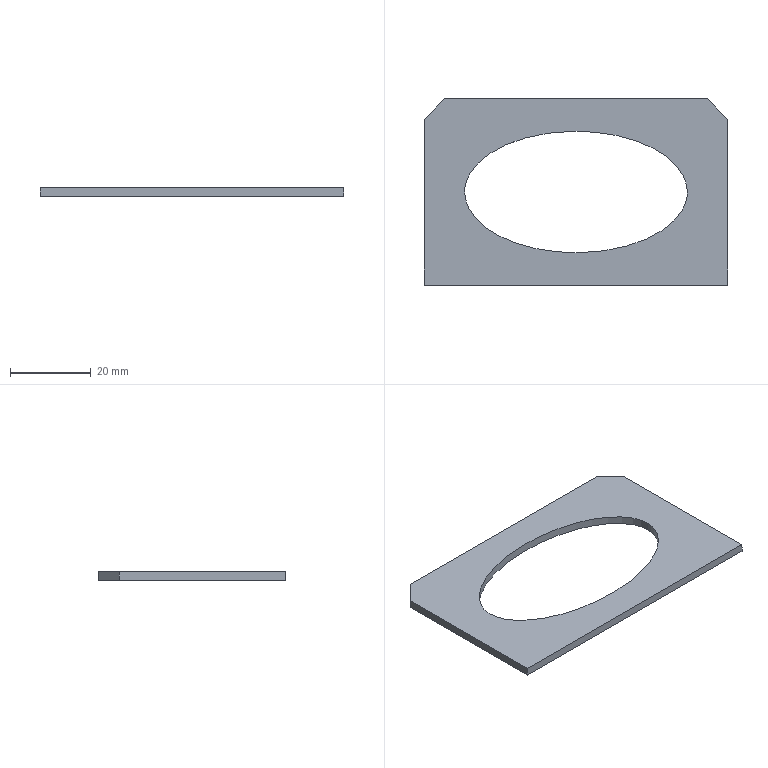Part | SolidWorks | features Chamfer 1, Cut 1, FlatPattern 1, SMBaseFlange 1, SheetMetal 1 | 1 solid | 10 faces | box 75 x 46 x 2 mm | volume 4258 mm3 | plane 8 | spline 2
STEP:
#1=CARTESIAN_POINT('',(27.5,0.,-2.));
#2=VERTEX_POINT('',#1);
#3=CARTESIAN_POINT('',(-27.5,0.,-2.));
#4=VERTEX_POINT('',#3);
#5=CARTESIAN_POINT('',(27.5,0.,-2.));
#6=CARTESIAN_POINT('',(27.5,30.,-2.));
#7=CARTESIAN_POINT('',(-27.5,30.,-2.));
#8=CARTESIAN_POINT('',(-27.5,0.,-2.));
#9=(BOUNDED_CURVE()B_SPLINE_CURVE(3,(#5,#6,#7,#8),.UNSPECIFIED.,.F.,.T.)B_SPLINE_CURVE_WITH_KNOTS((4,4),(3.142,6.283),.UNSPECIFIED.)CURVE()GEOMETRIC_REPRESENTATION_ITEM()RATIONAL_B_SPLINE_CURVE((1.,0.3333,0.3333,1.))REPRESENTATION_ITEM(''));
#10=EDGE_CURVE('',#2,#4,#9,.T.);
#11=ORIENTED_EDGE('',*,*,#10,.F.);
#12=CARTESIAN_POINT('',(27.5,0.,0.));
#13=VERTEX_POINT('',#12);
#14=CARTESIAN_POINT('',(27.5,0.,-2.));
#15=DIRECTION('',(0.,0.,1.));
#16=VECTOR('',#15,1000.);
#17=LINE('',#14,#16);
#18=EDGE_CURVE('',#2,#13,#17,.T.);
#19=ORIENTED_EDGE('',*,*,#18,.T.);
#20=CARTESIAN_POINT('',(-27.5,0.,0.));
#21=VERTEX_POINT('',#20);
#22=CARTESIAN_POINT('',(27.5,0.,0.));
#23=CARTESIAN_POINT('',(27.5,30.,0.));
#24=CARTESIAN_POINT('',(-27.5,30.,0.));
#25=CARTESIAN_POINT('',(-27.5,0.,0.));
#26=(BOUNDED_CURVE()B_SPLINE_CURVE(3,(#22,#23,#24,#25),.UNSPECIFIED.,.F.,.F.)B_SPLINE_CURVE_WITH_KNOTS((4,4),(3.142,6.283),.UNSPECIFIED.)CURVE()GEOMETRIC_REPRESENTATION_ITEM()RATIONAL_B_SPLINE_CURVE((1.,0.3333,0.3333,1.))REPRESENTATION_ITEM(''));
#27=EDGE_CURVE('',#13,#21,#26,.T.);
#28=ORIENTED_EDGE('',*,*,#27,.T.);
#29=CARTESIAN_POINT('',(-27.5,0.,-2.));
#30=DIRECTION('',(0.,0.,1.));
#31=VECTOR('',#30,1000.);
#32=LINE('',#29,#31);
#33=EDGE_CURVE('',#4,#21,#32,.T.);
#34=ORIENTED_EDGE('',*,*,#33,.F.);
#35=EDGE_LOOP('',(#11,#19,#28,#34));
#36=FACE_OUTER_BOUND('',#35,.T.);
#37=CARTESIAN_POINT('',(27.5,0.,-2.));
#38=CARTESIAN_POINT('',(27.5,0.,0.));
#39=CARTESIAN_POINT('',(27.5,30.,-2.));
#40=CARTESIAN_POINT('',(27.5,30.,0.));
#41=CARTESIAN_POINT('',(-27.5,30.,-2.));
#42=CARTESIAN_POINT('',(-27.5,30.,0.));
#43=CARTESIAN_POINT('',(-27.5,0.,-2.));
#44=CARTESIAN_POINT('',(-27.5,0.,0.));
#45=(BOUNDED_SURFACE()B_SPLINE_SURFACE(3,1,((#37,#38),(#39,#40),(#41,#42),(#43,#44)),.UNSPECIFIED.,.F.,.F.,.T.)B_SPLINE_SURFACE_WITH_KNOTS((4,4),(2,2),(0.,1.),(0.,1.),.UNSPECIFIED.)GEOMETRIC_REPRESENTATION_ITEM()RATIONAL_B_SPLINE_SURFACE(((1.,1.),(0.3333,0.3333),(0.3333,0.3333),(1.,1.)))REPRESENTATION_ITEM('')SURFACE());
#46=ADVANCED_FACE('',(#36),#45,.F.);
#47=CARTESIAN_POINT('',(37.5,-23.,-2.));
#48=VERTEX_POINT('',#47);
#49=CARTESIAN_POINT('',(37.5,18.,-2.));
#50=VERTEX_POINT('',#49);
#51=CARTESIAN_POINT('',(37.5,23.,-2.));
#52=DIRECTION('',(0.,1.,0.));
#53=VECTOR('',#52,1000.);
#54=LINE('',#51,#53);
#55=EDGE_CURVE('',#48,#50,#54,.T.);
#56=ORIENTED_EDGE('',*,*,#55,.T.);
#57=CARTESIAN_POINT('',(37.5,18.,0.));
#58=VERTEX_POINT('',#57);
#59=CARTESIAN_POINT('',(37.5,18.,-2.));
#60=DIRECTION('',(0.,0.,1.));
#61=VECTOR('',#60,1000.);
#62=LINE('',#59,#61);
#63=EDGE_CURVE('',#50,#58,#62,.T.);
#64=ORIENTED_EDGE('',*,*,#63,.T.);
#65=CARTESIAN_POINT('',(37.5,-23.,0.));
#66=VERTEX_POINT('',#65);
#67=CARTESIAN_POINT('',(37.5,23.,0.));
#68=DIRECTION('',(0.,1.,0.));
#69=VECTOR('',#68,1000.);
#70=LINE('',#67,#69);
#71=EDGE_CURVE('',#66,#58,#70,.T.);
#72=ORIENTED_EDGE('',*,*,#71,.F.);
#73=CARTESIAN_POINT('',(37.5,-23.,-2.));
#74=DIRECTION('',(0.,0.,1.));
#75=VECTOR('',#74,1000.);
#76=LINE('',#73,#75);
#77=EDGE_CURVE('',#48,#66,#76,.T.);
#78=ORIENTED_EDGE('',*,*,#77,.F.);
#79=EDGE_LOOP('',(#56,#64,#72,#78));
#80=FACE_OUTER_BOUND('',#79,.T.);
#81=CARTESIAN_POINT('',(37.5,23.,-2.));
#82=DIRECTION('',(1.,0.,0.));
#83=DIRECTION('',(0.,0.,-1.));
#84=AXIS2_PLACEMENT_3D('',#81,#82,#83);
#85=PLANE('',#84);
#86=ADVANCED_FACE('',(#80),#85,.T.);
#87=CARTESIAN_POINT('',(-37.5,-23.,0.));
#88=VERTEX_POINT('',#87);
#89=CARTESIAN_POINT('',(-37.5,-23.,0.));
#90=DIRECTION('',(1.,0.,0.));
#91=VECTOR('',#90,1000.);
#92=LINE('',#89,#91);
#93=EDGE_CURVE('',#88,#66,#92,.T.);
#94=ORIENTED_EDGE('',*,*,#93,.F.);
#95=CARTESIAN_POINT('',(-37.5,-23.,-2.));
#96=VERTEX_POINT('',#95);
#97=CARTESIAN_POINT('',(-37.5,-23.,-2.));
#98=DIRECTION('',(0.,0.,1.));
#99=VECTOR('',#98,1000.);
#100=LINE('',#97,#99);
#101=EDGE_CURVE('',#96,#88,#100,.T.);
#102=ORIENTED_EDGE('',*,*,#101,.F.);
#103=CARTESIAN_POINT('',(-37.5,-23.,-2.));
#104=DIRECTION('',(1.,0.,0.));
#105=VECTOR('',#104,1000.);
#106=LINE('',#103,#105);
#107=EDGE_CURVE('',#96,#48,#106,.T.);
#108=ORIENTED_EDGE('',*,*,#107,.T.);
#109=ORIENTED_EDGE('',*,*,#77,.T.);
#110=EDGE_LOOP('',(#94,#102,#108,#109));
#111=FACE_OUTER_BOUND('',#110,.T.);
#112=CARTESIAN_POINT('',(-37.5,-23.,-2.));
#113=DIRECTION('',(0.,-1.,0.));
#114=DIRECTION('',(0.,0.,-1.));
#115=AXIS2_PLACEMENT_3D('',#112,#113,#114);
#116=PLANE('',#115);
#117=ADVANCED_FACE('',(#111),#116,.T.);
#118=CARTESIAN_POINT('',(-37.5,18.,0.));
#119=VERTEX_POINT('',#118);
#120=CARTESIAN_POINT('',(-37.5,23.,0.));
#121=DIRECTION('',(0.,-1.,0.));
#122=VECTOR('',#121,1000.);
#123=LINE('',#120,#122);
#124=EDGE_CURVE('',#119,#88,#123,.T.);
#125=ORIENTED_EDGE('',*,*,#124,.F.);
#126=CARTESIAN_POINT('',(-37.5,18.,-2.));
#127=VERTEX_POINT('',#126);
#128=CARTESIAN_POINT('',(-37.5,18.,-2.));
#129=DIRECTION('',(0.,0.,-1.));
#130=VECTOR('',#129,1000.);
#131=LINE('',#128,#130);
#132=EDGE_CURVE('',#119,#127,#131,.T.);
#133=ORIENTED_EDGE('',*,*,#132,.T.);
#134=CARTESIAN_POINT('',(-37.5,23.,-2.));
#135=DIRECTION('',(0.,-1.,0.));
#136=VECTOR('',#135,1000.);
#137=LINE('',#134,#136);
#138=EDGE_CURVE('',#127,#96,#137,.T.);
#139=ORIENTED_EDGE('',*,*,#138,.T.);
#140=ORIENTED_EDGE('',*,*,#101,.T.);
#141=EDGE_LOOP('',(#125,#133,#139,#140));
#142=FACE_OUTER_BOUND('',#141,.T.);
#143=CARTESIAN_POINT('',(-37.5,23.,-2.));
#144=DIRECTION('',(-1.,0.,0.));
#145=DIRECTION('',(0.,-1.,0.));
#146=AXIS2_PLACEMENT_3D('',#143,#144,#145);
#147=PLANE('',#146);
#148=ADVANCED_FACE('',(#142),#147,.T.);
#149=CARTESIAN_POINT('',(32.5,23.,0.));
#150=VERTEX_POINT('',#149);
#151=CARTESIAN_POINT('',(-32.5,23.,0.));
#152=VERTEX_POINT('',#151);
#153=CARTESIAN_POINT('',(-37.5,23.,0.));
#154=DIRECTION('',(-1.,0.,0.));
#155=VECTOR('',#154,1000.);
#156=LINE('',#153,#155);
#157=EDGE_CURVE('',#150,#152,#156,.T.);
#158=ORIENTED_EDGE('',*,*,#157,.F.);
#159=CARTESIAN_POINT('',(32.5,23.,-2.));
#160=VERTEX_POINT('',#159);
#161=CARTESIAN_POINT('',(32.5,23.,-2.));
#162=DIRECTION('',(0.,0.,-1.));
#163=VECTOR('',#162,1000.);
#164=LINE('',#161,#163);
#165=EDGE_CURVE('',#150,#160,#164,.T.);
#166=ORIENTED_EDGE('',*,*,#165,.T.);
#167=CARTESIAN_POINT('',(-32.5,23.,-2.));
#168=VERTEX_POINT('',#167);
#169=CARTESIAN_POINT('',(-37.5,23.,-2.));
#170=DIRECTION('',(-1.,0.,0.));
#171=VECTOR('',#170,1000.);
#172=LINE('',#169,#171);
#173=EDGE_CURVE('',#160,#168,#172,.T.);
#174=ORIENTED_EDGE('',*,*,#173,.T.);
#175=CARTESIAN_POINT('',(-32.5,23.,-2.));
#176=DIRECTION('',(0.,0.,1.));
#177=VECTOR('',#176,1000.);
#178=LINE('',#175,#177);
#179=EDGE_CURVE('',#168,#152,#178,.T.);
#180=ORIENTED_EDGE('',*,*,#179,.T.);
#181=EDGE_LOOP('',(#158,#166,#174,#180));
#182=FACE_OUTER_BOUND('',#181,.T.);
#183=CARTESIAN_POINT('',(-37.5,23.,-2.));
#184=DIRECTION('',(0.,1.,0.));
#185=DIRECTION('',(0.,0.,1.));
#186=AXIS2_PLACEMENT_3D('',#183,#184,#185);
#187=PLANE('',#186);
#188=ADVANCED_FACE('',(#182),#187,.T.);
#189=CARTESIAN_POINT('',(-27.5,0.,-2.));
#190=CARTESIAN_POINT('',(-27.5,-30.,-2.));
#191=CARTESIAN_POINT('',(27.5,-30.,-2.));
#192=CARTESIAN_POINT('',(27.5,0.,-2.));
#193=(BOUNDED_CURVE()B_SPLINE_CURVE(3,(#189,#190,#191,#192),.UNSPECIFIED.,.F.,.F.)B_SPLINE_CURVE_WITH_KNOTS((4,4),(0.,3.142),.UNSPECIFIED.)CURVE()GEOMETRIC_REPRESENTATION_ITEM()RATIONAL_B_SPLINE_CURVE((1.,0.3333,0.3333,1.))REPRESENTATION_ITEM(''));
#194=EDGE_CURVE('',#4,#2,#193,.T.);
#195=ORIENTED_EDGE('',*,*,#194,.T.);
#196=ORIENTED_EDGE('',*,*,#10,.T.);
#197=EDGE_LOOP('',(#195,#196));
#198=FACE_BOUND('',#197,.T.);
#199=ORIENTED_EDGE('',*,*,#173,.F.);
#200=CARTESIAN_POINT('',(37.5,18.,-2.));
#201=DIRECTION('',(0.7071,-0.7071,0.));
#202=VECTOR('',#201,1000.);
#203=LINE('',#200,#202);
#204=EDGE_CURVE('',#160,#50,#203,.T.);
#205=ORIENTED_EDGE('',*,*,#204,.T.);
#206=ORIENTED_EDGE('',*,*,#55,.F.);
#207=ORIENTED_EDGE('',*,*,#107,.F.);
#208=ORIENTED_EDGE('',*,*,#138,.F.);
#209=CARTESIAN_POINT('',(-32.5,23.,-2.));
#210=DIRECTION('',(0.7071,0.7071,0.));
#211=VECTOR('',#210,1000.);
#212=LINE('',#209,#211);
#213=EDGE_CURVE('',#127,#168,#212,.T.);
#214=ORIENTED_EDGE('',*,*,#213,.T.);
#215=EDGE_LOOP('',(#199,#205,#206,#207,#208,#214));
#216=FACE_OUTER_BOUND('',#215,.T.);
#217=CARTESIAN_POINT('',(0.,0.,-2.));
#218=DIRECTION('',(0.,0.,1.));
#219=DIRECTION('',(1.,0.,0.));
#220=AXIS2_PLACEMENT_3D('',#217,#218,#219);
#221=PLANE('',#220);
#222=ADVANCED_FACE('',(#198,#216),#221,.F.);
#223=CARTESIAN_POINT('',(-27.5,0.,0.));
#224=CARTESIAN_POINT('',(-27.5,-30.,0.));
#225=CARTESIAN_POINT('',(27.5,-30.,0.));
#226=CARTESIAN_POINT('',(27.5,0.,0.));
#227=(BOUNDED_CURVE()B_SPLINE_CURVE(3,(#223,#224,#225,#226),.UNSPECIFIED.,.F.,.F.)B_SPLINE_CURVE_WITH_KNOTS((4,4),(0.,3.142),.UNSPECIFIED.)CURVE()GEOMETRIC_REPRESENTATION_ITEM()RATIONAL_B_SPLINE_CURVE((1.,0.3333,0.3333,1.))REPRESENTATION_ITEM(''));
#228=EDGE_CURVE('',#21,#13,#227,.T.);
#229=ORIENTED_EDGE('',*,*,#228,.F.);
#230=ORIENTED_EDGE('',*,*,#27,.F.);
#231=EDGE_LOOP('',(#229,#230));
#232=FACE_BOUND('',#231,.T.);
#233=ORIENTED_EDGE('',*,*,#71,.T.);
#234=CARTESIAN_POINT('',(27.75,27.75,0.));
#235=DIRECTION('',(-0.7071,0.7071,0.));
#236=VECTOR('',#235,1000.);
#237=LINE('',#234,#236);
#238=EDGE_CURVE('',#58,#150,#237,.T.);
#239=ORIENTED_EDGE('',*,*,#238,.T.);
#240=ORIENTED_EDGE('',*,*,#157,.T.);
#241=CARTESIAN_POINT('',(-27.75,27.75,0.));
#242=DIRECTION('',(-0.7071,-0.7071,0.));
#243=VECTOR('',#242,1000.);
#244=LINE('',#241,#243);
#245=EDGE_CURVE('',#152,#119,#244,.T.);
#246=ORIENTED_EDGE('',*,*,#245,.T.);
#247=ORIENTED_EDGE('',*,*,#124,.T.);
#248=ORIENTED_EDGE('',*,*,#93,.T.);
#249=EDGE_LOOP('',(#233,#239,#240,#246,#247,#248));
#250=FACE_OUTER_BOUND('',#249,.T.);
#251=CARTESIAN_POINT('',(0.,0.,0.));
#252=DIRECTION('',(0.,0.,1.));
#253=DIRECTION('',(1.,0.,0.));
#254=AXIS2_PLACEMENT_3D('',#251,#252,#253);
#255=PLANE('',#254);
#256=ADVANCED_FACE('',(#232,#250),#255,.T.);
#257=ORIENTED_EDGE('',*,*,#204,.F.);
#258=ORIENTED_EDGE('',*,*,#165,.F.);
#259=ORIENTED_EDGE('',*,*,#238,.F.);
#260=ORIENTED_EDGE('',*,*,#63,.F.);
#261=EDGE_LOOP('',(#257,#258,#259,#260));
#262=FACE_OUTER_BOUND('',#261,.T.);
#263=CARTESIAN_POINT('',(37.5,18.,-2.));
#264=DIRECTION('',(-0.7071,-0.7071,0.));
#265=DIRECTION('',(0.,0.,1.));
#266=AXIS2_PLACEMENT_3D('',#263,#264,#265);
#267=PLANE('',#266);
#268=ADVANCED_FACE('',(#262),#267,.F.);
#269=ORIENTED_EDGE('',*,*,#213,.F.);
#270=ORIENTED_EDGE('',*,*,#132,.F.);
#271=ORIENTED_EDGE('',*,*,#245,.F.);
#272=ORIENTED_EDGE('',*,*,#179,.F.);
#273=EDGE_LOOP('',(#269,#270,#271,#272));
#274=FACE_OUTER_BOUND('',#273,.T.);
#275=CARTESIAN_POINT('',(-32.5,23.,-2.));
#276=DIRECTION('',(0.7071,-0.7071,0.));
#277=DIRECTION('',(0.,0.,1.));
#278=AXIS2_PLACEMENT_3D('',#275,#276,#277);
#279=PLANE('',#278);
#280=ADVANCED_FACE('',(#274),#279,.F.);
#281=ORIENTED_EDGE('',*,*,#18,.F.);
#282=ORIENTED_EDGE('',*,*,#194,.F.);
#283=ORIENTED_EDGE('',*,*,#33,.T.);
#284=ORIENTED_EDGE('',*,*,#228,.T.);
#285=EDGE_LOOP('',(#281,#282,#283,#284));
#286=FACE_OUTER_BOUND('',#285,.T.);
#287=CARTESIAN_POINT('',(-27.5,0.,-2.));
#288=CARTESIAN_POINT('',(-27.5,0.,0.));
#289=CARTESIAN_POINT('',(-27.5,-30.,-2.));
#290=CARTESIAN_POINT('',(-27.5,-30.,0.));
#291=CARTESIAN_POINT('',(27.5,-30.,-2.));
#292=CARTESIAN_POINT('',(27.5,-30.,0.));
#293=CARTESIAN_POINT('',(27.5,0.,-2.));
#294=CARTESIAN_POINT('',(27.5,0.,0.));
#295=(BOUNDED_SURFACE()B_SPLINE_SURFACE(3,1,((#287,#288),(#289,#290),(#291,#292),(#293,#294)),.UNSPECIFIED.,.F.,.F.,.T.)B_SPLINE_SURFACE_WITH_KNOTS((4,4),(2,2),(0.,1.),(0.,1.),.UNSPECIFIED.)GEOMETRIC_REPRESENTATION_ITEM()RATIONAL_B_SPLINE_SURFACE(((1.,1.),(0.3333,0.3333),(0.3333,0.3333),(1.,1.)))REPRESENTATION_ITEM('')SURFACE());
#296=ADVANCED_FACE('',(#286),#295,.F.);
#297=CLOSED_SHELL('',(#46,#86,#117,#148,#188,#222,#256,#268,#280,#296));
#298=MANIFOLD_SOLID_BREP('',#297);
#299=CARTESIAN_POINT('',(0.,0.,0.));
#300=DIRECTION('',(0.,0.,1.));
#301=DIRECTION('',(1.,0.,0.));
#302=AXIS2_PLACEMENT_3D('',#299,#300,#301);
#303=(LENGTH_UNIT()NAMED_UNIT(*)SI_UNIT(.MILLI.,.METRE.));
#304=UNCERTAINTY_MEASURE_WITH_UNIT(LENGTH_MEASURE(0.00001),#303,'','');
#305=(NAMED_UNIT(*)PLANE_ANGLE_UNIT()SI_UNIT($,.RADIAN.));
#306=(NAMED_UNIT(*)SI_UNIT($,.STERADIAN.)SOLID_ANGLE_UNIT());
#307=(GEOMETRIC_REPRESENTATION_CONTEXT(3)GLOBAL_UNCERTAINTY_ASSIGNED_CONTEXT((#304))GLOBAL_UNIT_ASSIGNED_CONTEXT((#303,#305,#306))REPRESENTATION_CONTEXT('',''));
#308=ADVANCED_BREP_SHAPE_REPRESENTATION('',(#298,#302),#307);